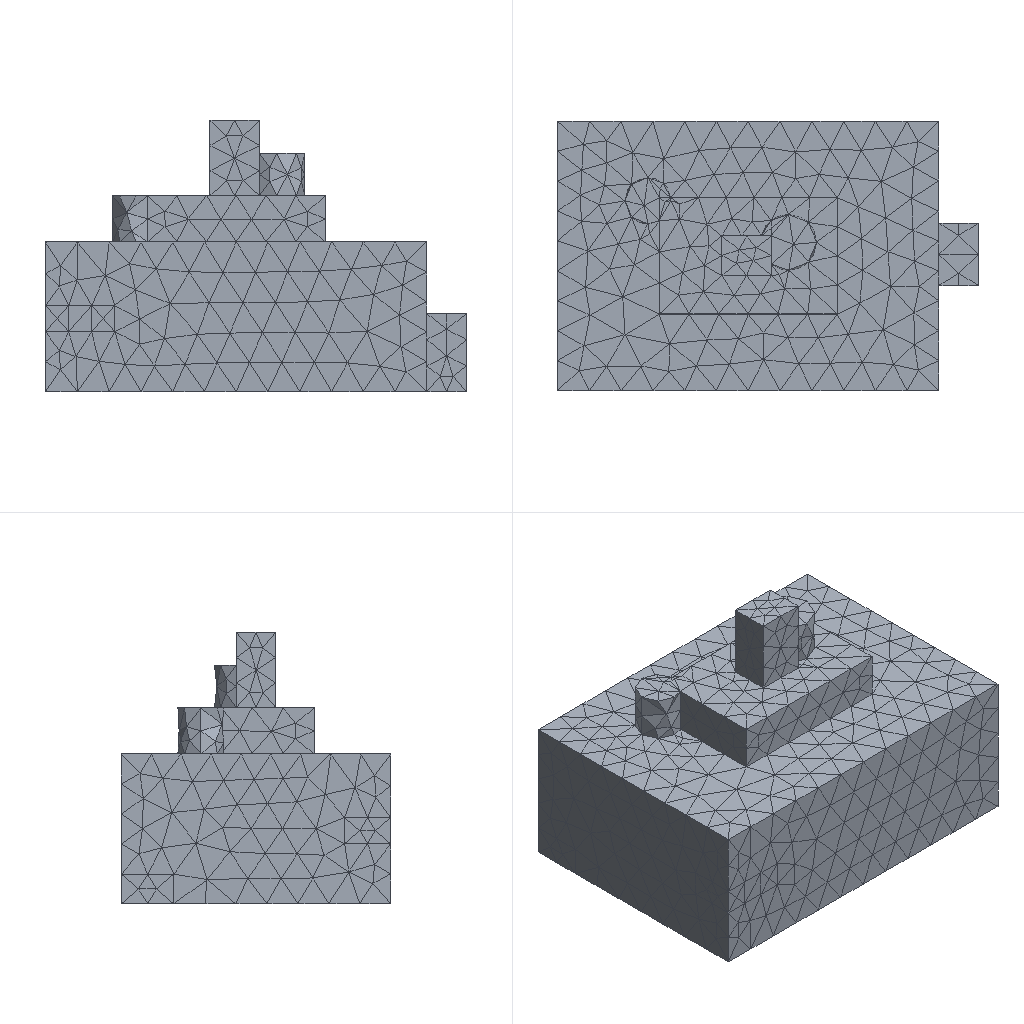Simulation study | ansys mapdl
Set-up summary:
category,name,step,type,value,unit,region
solver,ansys_mapdl
units,mm-N-s-tonne (MPa),,inferred,E=210000 density=
analysis,model,,static
mesh,nodes,,,9424
mesh,elements,,,5993
element_type,SOLID187,,,5993
material,mat 1,,E,210000
material,mat 1,,nu,0.3
load,,model,body load temp,,,all
load,,model,force,"1000 [dir=(0, 0, -1) n=278]",,node list
bc,,model,fixed,"[dofs=UX,UY,UZ n=9962]",,node list
Ansys APDL input file, long lists of numbers shortened:
/COM,ANSYS RELEASE 2026 R1           BUILD 26.1      UP20260202       09:09:04
/PREP7
/NOPR
/TITLE,2
ANTYPE, 0
*IF,_CDRDOFF,EQ,1,THEN     !if solid model was read in
_CDRDOFF=             !reset flag, numoffs already performed
*ELSE              !offset database for the following FE model
NUMOFF,NODE,     9424
NUMOFF,ELEM,     5993
NUMOFF,MAT ,        1
NUMOFF,TYPE,        1
*ENDIF
*SET,_RETURN ,  0.
*SET,_STATUS ,  0.
*SET,_UIQR   ,  278.
*SET,__FLOATPARAMETER__,  9424.
DOF,DELETE
ETBLOCK,        1,        1
(2i9,19a9)
        1      187        0        0        0        0        0        0        0        0        0        0        0        0        0        0        0        0        0        0        0
       -1
NBLOCK,6,SOLID,      9424,      9424
(3i9,6e21.13e3)
        1        0        0 7.0000000000000E+000 6.0000000000000E+000 8.2530000000000E+001
! (9423 more lines like these left out)
N,UNBL,LOC,       -1,
EBLOCK,19,SOLID,      5993,      5993
(19i10)
         1         1         1         1         0         0         0         0        10         0         1      2787      2788      2789        50      3457      3458      3459      3460
! (11985 more lines like these left out)
        -1
MPTEMP,UNBL, 1, 1,  0.    ,
MPDATA,UNBL, 1,EX  ,       1, 1,  210000.000    ,
MPTEMP,UNBL, 1, 1,  0.    ,
MPDATA,UNBL, 1,NUXY,       1, 1, 0.3    ,
MPTEMP,UNBL, 1, 1,  0.    ,
MPDATA,UNBL, 1,PRXY,       1, 1, 0.3    ,
EXTOPT,ATTR,      0,      0,      0
EXTOPT,ESIZE,  0,  0.
EXTOPT,ACLEAR,      0
TREF,  0.
IRLF,  0
BFUNIF,TEMP,_TINY
ACEL,  0.    ,  0.    ,  0.
OMEGA,  0.    ,  0.    ,  0.
DOMEGA,  0.    ,  0.    ,  0.
CGLOC,  0.    ,  0.    ,  0.
CGOMEGA,  0.    ,  0.    ,  0.
DCGOMG,  0.    ,  0.    ,  0.
KUSE,     0
TIME,  0.
ALPHAD,  0.
BETAD,  0.
DMPRAT,  0.
DMPSTR,  0.
CRPLIM, 0.1    ,   0
CRPLIM,  0.    ,   1
NCNV,     0, 1.000000000E+12,     0,  0.    ,  0.
NEQIT,     0
ERESX,DEFA
DBLOCK,      9962
(i9,a6,2(pg16.9))
      516  UX    0.00000000      0.00000000
! (9961 more lines like these left out)
       -1
FBLOCK,       278
(i9,a6,2(pg16.9))
        1  FZ   -3.59712230      0.00000000
! (277 more lines like these left out)
       -1
/GO
FINISH
Results summary:
result,analysis_type_db,,,static,unstated
result,n_sets,,,1,unstated
result,load_steps[0].set,load_step=1,,1,unstated
result,load_steps[0].substep,load_step=1,,1,unstated
result,load_steps[0].time,load_step=1,,1,unstated
result,load_steps[0].freq,load_step=1,,1,unstated
result,load_steps[0].max_usum,load_step=1,,0.0006577,unstated
result,load_steps[0].max_seqv,load_step=1,,4.828,unstated
result,load_steps[0].reaction_sum.FX,load_step=1,,-7.08376e-11,unstated
result,load_steps[0].reaction_sum.FY,load_step=1,,-2.14619e-11,unstated
result,load_steps[0].reaction_sum.FZ,load_step=1,,1000,unstated
result,load_steps[0].reaction_sum.MX,load_step=1,,0,unstated
result,load_steps[0].reaction_sum.MY,load_step=1,,0,unstated
result,load_steps[0].reaction_sum.MZ,load_step=1,,0,unstated
result,convergence,,,results present for all listed sets,unstated